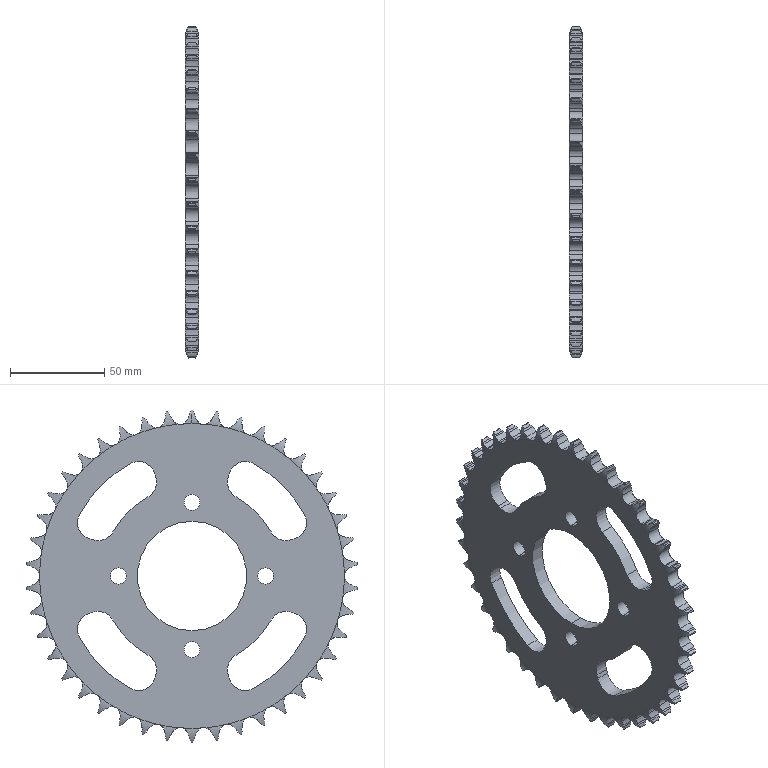Part | SolidWorks | features BaseBody 1 | 1 solid | 491 faces | box 7.28 x 175.563 x 176 mm | volume 107943 mm3 | cylinder 311 | plane 94 | torus 86 | commonest cylinder face diameters 12.099 x88 22.269 x88 8.653 x54 176 x43 18 x20 8.5 x8